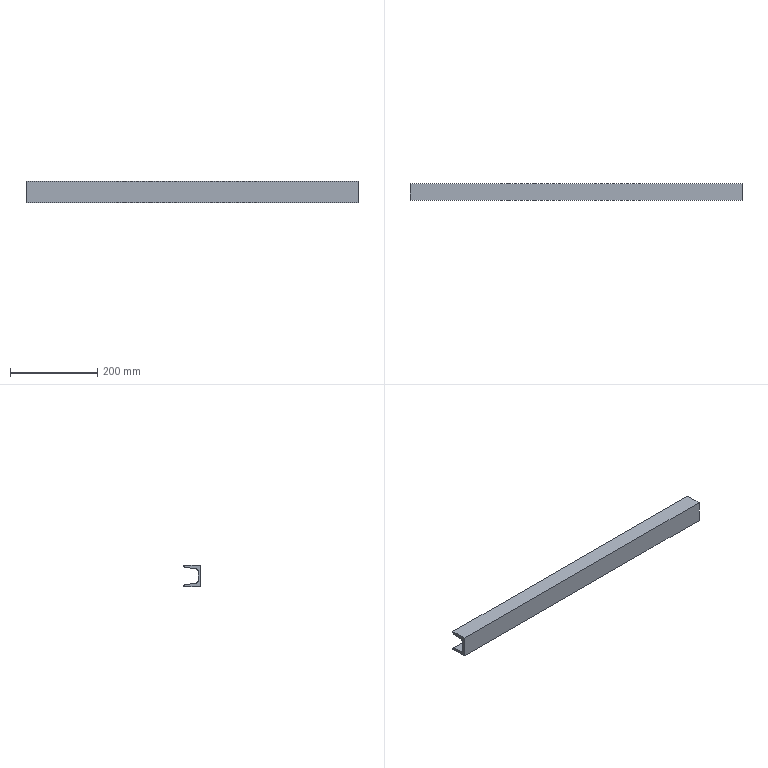Part | SolidWorks | features WeldMemberFeat 1, WeldmentFeature 1 | 1 solid | 14 faces | box 760 x 37 x 50 mm | volume 526149 mm3 | plane 10 | cylinder 4 | commonest cylinder face diameters 7 x2 14 x2
STEP:
#1=CARTESIAN_POINT('',(-380.,33.866,44.379));
#2=VERTEX_POINT('',#1);
#3=CARTESIAN_POINT('',(-380.,37.,47.859));
#4=VERTEX_POINT('',#3);
#5=CARTESIAN_POINT('',(-380.,33.5,47.859));
#6=DIRECTION('',(1.,0.,0.));
#7=DIRECTION('',(0.,1.,0.));
#8=AXIS2_PLACEMENT_3D('',#5,#6,#7);
#9=CIRCLE('',#8,3.5);
#10=EDGE_CURVE('',#2,#4,#9,.T.);
#11=ORIENTED_EDGE('',*,*,#10,.T.);
#12=CARTESIAN_POINT('',(380.,37.,47.859));
#13=VERTEX_POINT('',#12);
#14=CARTESIAN_POINT('',(380.,37.,47.859));
#15=DIRECTION('',(-1.,0.,0.));
#16=VECTOR('',#15,1000.);
#17=LINE('',#14,#16);
#18=EDGE_CURVE('',#13,#4,#17,.T.);
#19=ORIENTED_EDGE('',*,*,#18,.F.);
#20=CARTESIAN_POINT('',(380.,33.866,44.379));
#21=VERTEX_POINT('',#20);
#22=CARTESIAN_POINT('',(380.,33.5,47.859));
#23=DIRECTION('',(1.,0.,0.));
#24=DIRECTION('',(0.,1.,0.));
#25=AXIS2_PLACEMENT_3D('',#22,#23,#24);
#26=CIRCLE('',#25,3.5);
#27=EDGE_CURVE('',#21,#13,#26,.T.);
#28=ORIENTED_EDGE('',*,*,#27,.F.);
#29=CARTESIAN_POINT('',(380.,33.866,44.379));
#30=DIRECTION('',(-1.,0.,0.));
#31=VECTOR('',#30,1000.);
#32=LINE('',#29,#31);
#33=EDGE_CURVE('',#21,#2,#32,.T.);
#34=ORIENTED_EDGE('',*,*,#33,.T.);
#35=EDGE_LOOP('',(#11,#19,#28,#34));
#36=FACE_OUTER_BOUND('',#35,.T.);
#37=CARTESIAN_POINT('',(380.,33.5,47.859));
#38=DIRECTION('',(-1.,0.,0.));
#39=DIRECTION('',(0.,-1.,0.));
#40=AXIS2_PLACEMENT_3D('',#37,#38,#39);
#41=CYLINDRICAL_SURFACE('',#40,3.5);
#42=ADVANCED_FACE('',(#36),#41,.T.);
#43=CARTESIAN_POINT('',(-380.,37.,50.));
#44=VERTEX_POINT('',#43);
#45=CARTESIAN_POINT('',(-380.,37.,50.));
#46=DIRECTION('',(0.,0.,1.));
#47=VECTOR('',#46,1000.);
#48=LINE('',#45,#47);
#49=EDGE_CURVE('',#4,#44,#48,.T.);
#50=ORIENTED_EDGE('',*,*,#49,.T.);
#51=CARTESIAN_POINT('',(380.,37.,50.));
#52=VERTEX_POINT('',#51);
#53=CARTESIAN_POINT('',(380.,37.,50.));
#54=DIRECTION('',(-1.,0.,0.));
#55=VECTOR('',#54,1000.);
#56=LINE('',#53,#55);
#57=EDGE_CURVE('',#52,#44,#56,.T.);
#58=ORIENTED_EDGE('',*,*,#57,.F.);
#59=CARTESIAN_POINT('',(380.,37.,50.));
#60=DIRECTION('',(0.,0.,1.));
#61=VECTOR('',#60,1000.);
#62=LINE('',#59,#61);
#63=EDGE_CURVE('',#13,#52,#62,.T.);
#64=ORIENTED_EDGE('',*,*,#63,.F.);
#65=ORIENTED_EDGE('',*,*,#18,.T.);
#66=EDGE_LOOP('',(#50,#58,#64,#65));
#67=FACE_OUTER_BOUND('',#66,.T.);
#68=CARTESIAN_POINT('',(380.,37.,50.));
#69=DIRECTION('',(0.,-1.,0.));
#70=DIRECTION('',(1.,0.,0.));
#71=AXIS2_PLACEMENT_3D('',#68,#69,#70);
#72=PLANE('',#71);
#73=ADVANCED_FACE('',(#67),#72,.F.);
#74=CARTESIAN_POINT('',(-380.,0.,50.));
#75=VERTEX_POINT('',#74);
#76=CARTESIAN_POINT('',(-380.,37.,50.));
#77=DIRECTION('',(0.,-1.,0.));
#78=VECTOR('',#77,1000.);
#79=LINE('',#76,#78);
#80=EDGE_CURVE('',#44,#75,#79,.T.);
#81=ORIENTED_EDGE('',*,*,#80,.T.);
#82=CARTESIAN_POINT('',(380.,0.,50.));
#83=VERTEX_POINT('',#82);
#84=CARTESIAN_POINT('',(380.,0.,50.));
#85=DIRECTION('',(-1.,0.,0.));
#86=VECTOR('',#85,1000.);
#87=LINE('',#84,#86);
#88=EDGE_CURVE('',#83,#75,#87,.T.);
#89=ORIENTED_EDGE('',*,*,#88,.F.);
#90=CARTESIAN_POINT('',(380.,37.,50.));
#91=DIRECTION('',(0.,-1.,0.));
#92=VECTOR('',#91,1000.);
#93=LINE('',#90,#92);
#94=EDGE_CURVE('',#52,#83,#93,.T.);
#95=ORIENTED_EDGE('',*,*,#94,.F.);
#96=ORIENTED_EDGE('',*,*,#57,.T.);
#97=EDGE_LOOP('',(#81,#89,#95,#96));
#98=FACE_OUTER_BOUND('',#97,.T.);
#99=CARTESIAN_POINT('',(380.,37.,50.));
#100=DIRECTION('',(0.,0.,-1.));
#101=DIRECTION('',(0.,1.,0.));
#102=AXIS2_PLACEMENT_3D('',#99,#100,#101);
#103=PLANE('',#102);
#104=ADVANCED_FACE('',(#98),#103,.F.);
#105=CARTESIAN_POINT('',(-380.,0.,0.));
#106=VERTEX_POINT('',#105);
#107=CARTESIAN_POINT('',(-380.,0.,50.));
#108=DIRECTION('',(0.,0.,-1.));
#109=VECTOR('',#108,1000.);
#110=LINE('',#107,#109);
#111=EDGE_CURVE('',#75,#106,#110,.T.);
#112=ORIENTED_EDGE('',*,*,#111,.T.);
#113=CARTESIAN_POINT('',(380.,0.,0.));
#114=VERTEX_POINT('',#113);
#115=CARTESIAN_POINT('',(380.,0.,0.));
#116=DIRECTION('',(-1.,0.,0.));
#117=VECTOR('',#116,1000.);
#118=LINE('',#115,#117);
#119=EDGE_CURVE('',#114,#106,#118,.T.);
#120=ORIENTED_EDGE('',*,*,#119,.F.);
#121=CARTESIAN_POINT('',(380.,0.,50.));
#122=DIRECTION('',(0.,0.,-1.));
#123=VECTOR('',#122,1000.);
#124=LINE('',#121,#123);
#125=EDGE_CURVE('',#83,#114,#124,.T.);
#126=ORIENTED_EDGE('',*,*,#125,.F.);
#127=ORIENTED_EDGE('',*,*,#88,.T.);
#128=EDGE_LOOP('',(#112,#120,#126,#127));
#129=FACE_OUTER_BOUND('',#128,.T.);
#130=CARTESIAN_POINT('',(380.,0.,50.));
#131=DIRECTION('',(0.,1.,0.));
#132=DIRECTION('',(-1.,0.,0.));
#133=AXIS2_PLACEMENT_3D('',#130,#131,#132);
#134=PLANE('',#133);
#135=ADVANCED_FACE('',(#129),#134,.F.);
#136=CARTESIAN_POINT('',(-380.,37.,0.));
#137=VERTEX_POINT('',#136);
#138=CARTESIAN_POINT('',(-380.,37.,0.));
#139=DIRECTION('',(0.,1.,0.));
#140=VECTOR('',#139,1000.);
#141=LINE('',#138,#140);
#142=EDGE_CURVE('',#106,#137,#141,.T.);
#143=ORIENTED_EDGE('',*,*,#142,.T.);
#144=CARTESIAN_POINT('',(380.,37.,0.));
#145=VERTEX_POINT('',#144);
#146=CARTESIAN_POINT('',(380.,37.,0.));
#147=DIRECTION('',(-1.,0.,0.));
#148=VECTOR('',#147,1000.);
#149=LINE('',#146,#148);
#150=EDGE_CURVE('',#145,#137,#149,.T.);
#151=ORIENTED_EDGE('',*,*,#150,.F.);
#152=CARTESIAN_POINT('',(380.,37.,0.));
#153=DIRECTION('',(0.,1.,0.));
#154=VECTOR('',#153,1000.);
#155=LINE('',#152,#154);
#156=EDGE_CURVE('',#114,#145,#155,.T.);
#157=ORIENTED_EDGE('',*,*,#156,.F.);
#158=ORIENTED_EDGE('',*,*,#119,.T.);
#159=EDGE_LOOP('',(#143,#151,#157,#158));
#160=FACE_OUTER_BOUND('',#159,.T.);
#161=CARTESIAN_POINT('',(380.,37.,0.));
#162=DIRECTION('',(0.,0.,1.));
#163=DIRECTION('',(0.,-1.,0.));
#164=AXIS2_PLACEMENT_3D('',#161,#162,#163);
#165=PLANE('',#164);
#166=ADVANCED_FACE('',(#160),#165,.F.);
#167=CARTESIAN_POINT('',(-380.,37.,2.141));
#168=VERTEX_POINT('',#167);
#169=CARTESIAN_POINT('',(-380.,37.,0.));
#170=DIRECTION('',(0.,0.,1.));
#171=VECTOR('',#170,1000.);
#172=LINE('',#169,#171);
#173=EDGE_CURVE('',#137,#168,#172,.T.);
#174=ORIENTED_EDGE('',*,*,#173,.T.);
#175=CARTESIAN_POINT('',(380.,37.,2.141));
#176=VERTEX_POINT('',#175);
#177=CARTESIAN_POINT('',(380.,37.,2.141));
#178=DIRECTION('',(-1.,0.,0.));
#179=VECTOR('',#178,1000.);
#180=LINE('',#177,#179);
#181=EDGE_CURVE('',#176,#168,#180,.T.);
#182=ORIENTED_EDGE('',*,*,#181,.F.);
#183=CARTESIAN_POINT('',(380.,37.,0.));
#184=DIRECTION('',(0.,0.,1.));
#185=VECTOR('',#184,1000.);
#186=LINE('',#183,#185);
#187=EDGE_CURVE('',#145,#176,#186,.T.);
#188=ORIENTED_EDGE('',*,*,#187,.F.);
#189=ORIENTED_EDGE('',*,*,#150,.T.);
#190=EDGE_LOOP('',(#174,#182,#188,#189));
#191=FACE_OUTER_BOUND('',#190,.T.);
#192=CARTESIAN_POINT('',(380.,37.,0.));
#193=DIRECTION('',(0.,-1.,0.));
#194=DIRECTION('',(1.,0.,0.));
#195=AXIS2_PLACEMENT_3D('',#192,#193,#194);
#196=PLANE('',#195);
#197=ADVANCED_FACE('',(#191),#196,.F.);
#198=CARTESIAN_POINT('',(-380.,33.866,5.621));
#199=VERTEX_POINT('',#198);
#200=CARTESIAN_POINT('',(-380.,33.5,2.141));
#201=DIRECTION('',(1.,0.,0.));
#202=DIRECTION('',(0.,-1.,0.));
#203=AXIS2_PLACEMENT_3D('',#200,#201,#202);
#204=CIRCLE('',#203,3.5);
#205=EDGE_CURVE('',#168,#199,#204,.T.);
#206=ORIENTED_EDGE('',*,*,#205,.T.);
#207=CARTESIAN_POINT('',(380.,33.866,5.621));
#208=VERTEX_POINT('',#207);
#209=CARTESIAN_POINT('',(380.,33.866,5.621));
#210=DIRECTION('',(-1.,0.,0.));
#211=VECTOR('',#210,1000.);
#212=LINE('',#209,#211);
#213=EDGE_CURVE('',#208,#199,#212,.T.);
#214=ORIENTED_EDGE('',*,*,#213,.F.);
#215=CARTESIAN_POINT('',(380.,33.5,2.141));
#216=DIRECTION('',(1.,0.,0.));
#217=DIRECTION('',(0.,-1.,0.));
#218=AXIS2_PLACEMENT_3D('',#215,#216,#217);
#219=CIRCLE('',#218,3.5);
#220=EDGE_CURVE('',#176,#208,#219,.T.);
#221=ORIENTED_EDGE('',*,*,#220,.F.);
#222=ORIENTED_EDGE('',*,*,#181,.T.);
#223=EDGE_LOOP('',(#206,#214,#221,#222));
#224=FACE_OUTER_BOUND('',#223,.T.);
#225=CARTESIAN_POINT('',(380.,33.5,2.141));
#226=DIRECTION('',(-1.,0.,0.));
#227=DIRECTION('',(0.,-1.,0.));
#228=AXIS2_PLACEMENT_3D('',#225,#226,#227);
#229=CYLINDRICAL_SURFACE('',#228,3.5);
#230=ADVANCED_FACE('',(#224),#229,.T.);
#231=CARTESIAN_POINT('',(-380.,10.768,8.049));
#232=VERTEX_POINT('',#231);
#233=CARTESIAN_POINT('',(-380.,10.768,8.049));
#234=DIRECTION('',(0.,-0.9945,0.1045));
#235=VECTOR('',#234,1000.);
#236=LINE('',#233,#235);
#237=EDGE_CURVE('',#199,#232,#236,.T.);
#238=ORIENTED_EDGE('',*,*,#237,.T.);
#239=CARTESIAN_POINT('',(380.,10.768,8.049));
#240=VERTEX_POINT('',#239);
#241=CARTESIAN_POINT('',(380.,10.768,8.049));
#242=DIRECTION('',(-1.,0.,0.));
#243=VECTOR('',#242,1000.);
#244=LINE('',#241,#243);
#245=EDGE_CURVE('',#240,#232,#244,.T.);
#246=ORIENTED_EDGE('',*,*,#245,.F.);
#247=CARTESIAN_POINT('',(380.,10.768,8.049));
#248=DIRECTION('',(0.,-0.9945,0.1045));
#249=VECTOR('',#248,1000.);
#250=LINE('',#247,#249);
#251=EDGE_CURVE('',#208,#240,#250,.T.);
#252=ORIENTED_EDGE('',*,*,#251,.F.);
#253=ORIENTED_EDGE('',*,*,#213,.T.);
#254=EDGE_LOOP('',(#238,#246,#252,#253));
#255=FACE_OUTER_BOUND('',#254,.T.);
#256=CARTESIAN_POINT('',(380.,10.768,8.049));
#257=DIRECTION('',(0.,-0.1045,-0.9945));
#258=DIRECTION('',(0.,0.9945,-0.1045));
#259=AXIS2_PLACEMENT_3D('',#256,#257,#258);
#260=PLANE('',#259);
#261=ADVANCED_FACE('',(#255),#260,.F.);
#262=CARTESIAN_POINT('',(-380.,4.5,15.011));
#263=VERTEX_POINT('',#262);
#264=CARTESIAN_POINT('',(-380.,11.5,15.011));
#265=DIRECTION('',(-1.,0.,0.));
#266=DIRECTION('',(0.,1.,0.));
#267=AXIS2_PLACEMENT_3D('',#264,#265,#266);
#268=CIRCLE('',#267,7.);
#269=EDGE_CURVE('',#232,#263,#268,.T.);
#270=ORIENTED_EDGE('',*,*,#269,.T.);
#271=CARTESIAN_POINT('',(380.,4.5,15.011));
#272=VERTEX_POINT('',#271);
#273=CARTESIAN_POINT('',(380.,4.5,15.011));
#274=DIRECTION('',(-1.,0.,0.));
#275=VECTOR('',#274,1000.);
#276=LINE('',#273,#275);
#277=EDGE_CURVE('',#272,#263,#276,.T.);
#278=ORIENTED_EDGE('',*,*,#277,.F.);
#279=CARTESIAN_POINT('',(380.,11.5,15.011));
#280=DIRECTION('',(-1.,0.,0.));
#281=DIRECTION('',(0.,1.,0.));
#282=AXIS2_PLACEMENT_3D('',#279,#280,#281);
#283=CIRCLE('',#282,7.);
#284=EDGE_CURVE('',#240,#272,#283,.T.);
#285=ORIENTED_EDGE('',*,*,#284,.F.);
#286=ORIENTED_EDGE('',*,*,#245,.T.);
#287=EDGE_LOOP('',(#270,#278,#285,#286));
#288=FACE_OUTER_BOUND('',#287,.T.);
#289=CARTESIAN_POINT('',(380.,11.5,15.011));
#290=DIRECTION('',(-1.,0.,0.));
#291=DIRECTION('',(0.,-1.,0.));
#292=AXIS2_PLACEMENT_3D('',#289,#290,#291);
#293=CYLINDRICAL_SURFACE('',#292,7.);
#294=ADVANCED_FACE('',(#288),#293,.F.);
#295=CARTESIAN_POINT('',(-380.,4.5,34.989));
#296=VERTEX_POINT('',#295);
#297=CARTESIAN_POINT('',(-380.,4.5,34.989));
#298=DIRECTION('',(0.,0.,1.));
#299=VECTOR('',#298,1000.);
#300=LINE('',#297,#299);
#301=EDGE_CURVE('',#263,#296,#300,.T.);
#302=ORIENTED_EDGE('',*,*,#301,.T.);
#303=CARTESIAN_POINT('',(380.,4.5,34.989));
#304=VERTEX_POINT('',#303);
#305=CARTESIAN_POINT('',(380.,4.5,34.989));
#306=DIRECTION('',(-1.,0.,0.));
#307=VECTOR('',#306,1000.);
#308=LINE('',#305,#307);
#309=EDGE_CURVE('',#304,#296,#308,.T.);
#310=ORIENTED_EDGE('',*,*,#309,.F.);
#311=CARTESIAN_POINT('',(380.,4.5,34.989));
#312=DIRECTION('',(0.,0.,1.));
#313=VECTOR('',#312,1000.);
#314=LINE('',#311,#313);
#315=EDGE_CURVE('',#272,#304,#314,.T.);
#316=ORIENTED_EDGE('',*,*,#315,.F.);
#317=ORIENTED_EDGE('',*,*,#277,.T.);
#318=EDGE_LOOP('',(#302,#310,#316,#317));
#319=FACE_OUTER_BOUND('',#318,.T.);
#320=CARTESIAN_POINT('',(380.,4.5,34.989));
#321=DIRECTION('',(0.,-1.,0.));
#322=DIRECTION('',(1.,0.,0.));
#323=AXIS2_PLACEMENT_3D('',#320,#321,#322);
#324=PLANE('',#323);
#325=ADVANCED_FACE('',(#319),#324,.F.);
#326=CARTESIAN_POINT('',(-380.,10.768,41.951));
#327=VERTEX_POINT('',#326);
#328=CARTESIAN_POINT('',(-380.,11.5,34.989));
#329=DIRECTION('',(-1.,0.,0.));
#330=DIRECTION('',(0.,-1.,0.));
#331=AXIS2_PLACEMENT_3D('',#328,#329,#330);
#332=CIRCLE('',#331,7.);
#333=EDGE_CURVE('',#296,#327,#332,.T.);
#334=ORIENTED_EDGE('',*,*,#333,.T.);
#335=CARTESIAN_POINT('',(380.,10.768,41.951));
#336=VERTEX_POINT('',#335);
#337=CARTESIAN_POINT('',(380.,10.768,41.951));
#338=DIRECTION('',(-1.,0.,0.));
#339=VECTOR('',#338,1000.);
#340=LINE('',#337,#339);
#341=EDGE_CURVE('',#336,#327,#340,.T.);
#342=ORIENTED_EDGE('',*,*,#341,.F.);
#343=CARTESIAN_POINT('',(380.,11.5,34.989));
#344=DIRECTION('',(-1.,0.,0.));
#345=DIRECTION('',(0.,-1.,0.));
#346=AXIS2_PLACEMENT_3D('',#343,#344,#345);
#347=CIRCLE('',#346,7.);
#348=EDGE_CURVE('',#304,#336,#347,.T.);
#349=ORIENTED_EDGE('',*,*,#348,.F.);
#350=ORIENTED_EDGE('',*,*,#309,.T.);
#351=EDGE_LOOP('',(#334,#342,#349,#350));
#352=FACE_OUTER_BOUND('',#351,.T.);
#353=CARTESIAN_POINT('',(380.,11.5,34.989));
#354=DIRECTION('',(-1.,0.,0.));
#355=DIRECTION('',(0.,-1.,0.));
#356=AXIS2_PLACEMENT_3D('',#353,#354,#355);
#357=CYLINDRICAL_SURFACE('',#356,7.);
#358=ADVANCED_FACE('',(#352),#357,.F.);
#359=CARTESIAN_POINT('',(-380.,10.768,41.951));
#360=DIRECTION('',(0.,0.9945,0.1045));
#361=VECTOR('',#360,1000.);
#362=LINE('',#359,#361);
#363=EDGE_CURVE('',#327,#2,#362,.T.);
#364=ORIENTED_EDGE('',*,*,#363,.T.);
#365=ORIENTED_EDGE('',*,*,#33,.F.);
#366=CARTESIAN_POINT('',(380.,10.768,41.951));
#367=DIRECTION('',(0.,0.9945,0.1045));
#368=VECTOR('',#367,1000.);
#369=LINE('',#366,#368);
#370=EDGE_CURVE('',#336,#21,#369,.T.);
#371=ORIENTED_EDGE('',*,*,#370,.F.);
#372=ORIENTED_EDGE('',*,*,#341,.T.);
#373=EDGE_LOOP('',(#364,#365,#371,#372));
#374=FACE_OUTER_BOUND('',#373,.T.);
#375=CARTESIAN_POINT('',(380.,10.768,41.951));
#376=DIRECTION('',(0.,-0.1045,0.9945));
#377=DIRECTION('',(0.,-0.9945,-0.1045));
#378=AXIS2_PLACEMENT_3D('',#375,#376,#377);
#379=PLANE('',#378);
#380=ADVANCED_FACE('',(#374),#379,.F.);
#381=ORIENTED_EDGE('',*,*,#27,.T.);
#382=ORIENTED_EDGE('',*,*,#63,.T.);
#383=ORIENTED_EDGE('',*,*,#94,.T.);
#384=ORIENTED_EDGE('',*,*,#125,.T.);
#385=ORIENTED_EDGE('',*,*,#156,.T.);
#386=ORIENTED_EDGE('',*,*,#187,.T.);
#387=ORIENTED_EDGE('',*,*,#220,.T.);
#388=ORIENTED_EDGE('',*,*,#251,.T.);
#389=ORIENTED_EDGE('',*,*,#284,.T.);
#390=ORIENTED_EDGE('',*,*,#315,.T.);
#391=ORIENTED_EDGE('',*,*,#348,.T.);
#392=ORIENTED_EDGE('',*,*,#370,.T.);
#393=EDGE_LOOP('',(#381,#382,#383,#384,#385,#386,#387,#388,#389,#390,#391,#392));
#394=FACE_OUTER_BOUND('',#393,.T.);
#395=CARTESIAN_POINT('',(380.,33.5,47.859));
#396=DIRECTION('',(1.,0.,0.));
#397=DIRECTION('',(0.,1.,0.));
#398=AXIS2_PLACEMENT_3D('',#395,#396,#397);
#399=PLANE('',#398);
#400=ADVANCED_FACE('',(#394),#399,.T.);
#401=ORIENTED_EDGE('',*,*,#10,.F.);
#402=ORIENTED_EDGE('',*,*,#363,.F.);
#403=ORIENTED_EDGE('',*,*,#333,.F.);
#404=ORIENTED_EDGE('',*,*,#301,.F.);
#405=ORIENTED_EDGE('',*,*,#269,.F.);
#406=ORIENTED_EDGE('',*,*,#237,.F.);
#407=ORIENTED_EDGE('',*,*,#205,.F.);
#408=ORIENTED_EDGE('',*,*,#173,.F.);
#409=ORIENTED_EDGE('',*,*,#142,.F.);
#410=ORIENTED_EDGE('',*,*,#111,.F.);
#411=ORIENTED_EDGE('',*,*,#80,.F.);
#412=ORIENTED_EDGE('',*,*,#49,.F.);
#413=EDGE_LOOP('',(#401,#402,#403,#404,#405,#406,#407,#408,#409,#410,#411,#412));
#414=FACE_OUTER_BOUND('',#413,.T.);
#415=CARTESIAN_POINT('',(-380.,33.5,47.859));
#416=DIRECTION('',(1.,0.,0.));
#417=DIRECTION('',(0.,1.,0.));
#418=AXIS2_PLACEMENT_3D('',#415,#416,#417);
#419=PLANE('',#418);
#420=ADVANCED_FACE('',(#414),#419,.F.);
#421=CLOSED_SHELL('',(#42,#73,#104,#135,#166,#197,#230,#261,#294,#325,#358,#380,#400,#420));
#422=MANIFOLD_SOLID_BREP('',#421);
#423=CARTESIAN_POINT('',(0.,0.,0.));
#424=DIRECTION('',(0.,0.,1.));
#425=DIRECTION('',(1.,0.,0.));
#426=AXIS2_PLACEMENT_3D('',#423,#424,#425);
#427=(LENGTH_UNIT()NAMED_UNIT(*)SI_UNIT(.MILLI.,.METRE.));
#428=UNCERTAINTY_MEASURE_WITH_UNIT(LENGTH_MEASURE(0.00001),#427,'','');
#429=(NAMED_UNIT(*)PLANE_ANGLE_UNIT()SI_UNIT($,.RADIAN.));
#430=(NAMED_UNIT(*)SI_UNIT($,.STERADIAN.)SOLID_ANGLE_UNIT());
#431=(GEOMETRIC_REPRESENTATION_CONTEXT(3)GLOBAL_UNCERTAINTY_ASSIGNED_CONTEXT((#428))GLOBAL_UNIT_ASSIGNED_CONTEXT((#427,#429,#430))REPRESENTATION_CONTEXT('',''));
#432=ADVANCED_BREP_SHAPE_REPRESENTATION('',(#422,#426),#431);